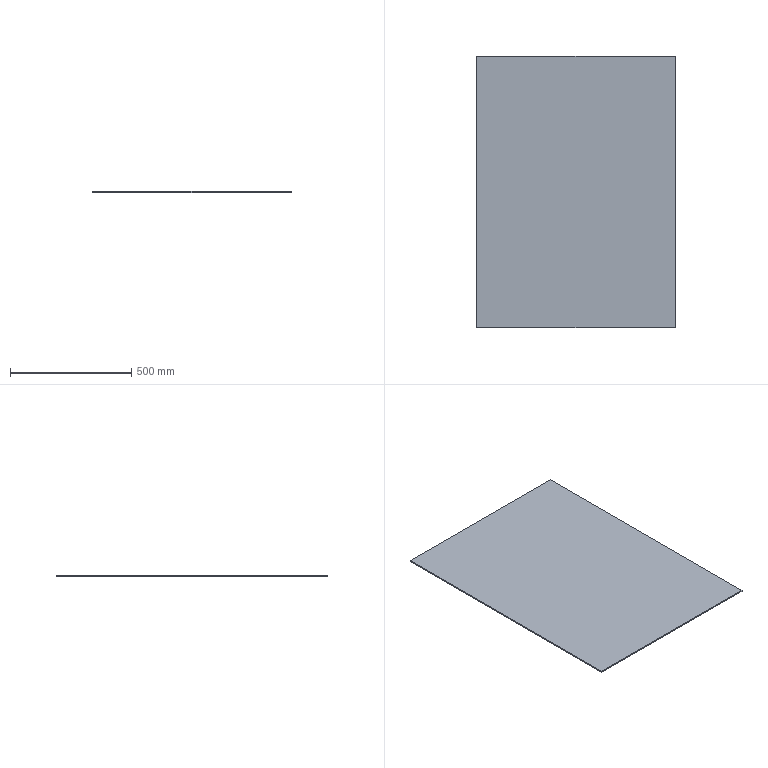Part | SolidWorks | features Extrusion 1 | 1 solid | 6 faces | box 818 x 1119 x 5 mm | volume 4576710 mm3 | plane 6
STEP:
#1=CARTESIAN_POINT('',(409.,-559.5,0.));
#2=VERTEX_POINT('',#1);
#3=CARTESIAN_POINT('',(409.,559.5,0.));
#4=VERTEX_POINT('',#3);
#5=CARTESIAN_POINT('',(409.,559.5,0.));
#6=DIRECTION('',(0.,1.,0.));
#7=VECTOR('',#6,1000.);
#8=LINE('',#5,#7);
#9=EDGE_CURVE('',#2,#4,#8,.T.);
#10=ORIENTED_EDGE('',*,*,#9,.T.);
#11=CARTESIAN_POINT('',(409.,559.5,5.));
#12=VERTEX_POINT('',#11);
#13=CARTESIAN_POINT('',(409.,559.5,5.));
#14=DIRECTION('',(0.,0.,-1.));
#15=VECTOR('',#14,1000.);
#16=LINE('',#13,#15);
#17=EDGE_CURVE('',#12,#4,#16,.T.);
#18=ORIENTED_EDGE('',*,*,#17,.F.);
#19=CARTESIAN_POINT('',(409.,-559.5,5.));
#20=VERTEX_POINT('',#19);
#21=CARTESIAN_POINT('',(409.,559.5,5.));
#22=DIRECTION('',(0.,1.,0.));
#23=VECTOR('',#22,1000.);
#24=LINE('',#21,#23);
#25=EDGE_CURVE('',#20,#12,#24,.T.);
#26=ORIENTED_EDGE('',*,*,#25,.F.);
#27=CARTESIAN_POINT('',(409.,-559.5,5.));
#28=DIRECTION('',(0.,0.,-1.));
#29=VECTOR('',#28,1000.);
#30=LINE('',#27,#29);
#31=EDGE_CURVE('',#20,#2,#30,.T.);
#32=ORIENTED_EDGE('',*,*,#31,.T.);
#33=EDGE_LOOP('',(#10,#18,#26,#32));
#34=FACE_OUTER_BOUND('',#33,.T.);
#35=CARTESIAN_POINT('',(409.,559.5,5.));
#36=DIRECTION('',(-1.,0.,0.));
#37=DIRECTION('',(0.,0.,1.));
#38=AXIS2_PLACEMENT_3D('',#35,#36,#37);
#39=PLANE('',#38);
#40=ADVANCED_FACE('',(#34),#39,.F.);
#41=CARTESIAN_POINT('',(-409.,559.5,0.));
#42=VERTEX_POINT('',#41);
#43=CARTESIAN_POINT('',(-409.,559.5,0.));
#44=DIRECTION('',(-1.,0.,0.));
#45=VECTOR('',#44,1000.);
#46=LINE('',#43,#45);
#47=EDGE_CURVE('',#4,#42,#46,.T.);
#48=ORIENTED_EDGE('',*,*,#47,.T.);
#49=CARTESIAN_POINT('',(-409.,559.5,5.));
#50=VERTEX_POINT('',#49);
#51=CARTESIAN_POINT('',(-409.,559.5,5.));
#52=DIRECTION('',(0.,0.,-1.));
#53=VECTOR('',#52,1000.);
#54=LINE('',#51,#53);
#55=EDGE_CURVE('',#50,#42,#54,.T.);
#56=ORIENTED_EDGE('',*,*,#55,.F.);
#57=CARTESIAN_POINT('',(-409.,559.5,5.));
#58=DIRECTION('',(-1.,0.,0.));
#59=VECTOR('',#58,1000.);
#60=LINE('',#57,#59);
#61=EDGE_CURVE('',#12,#50,#60,.T.);
#62=ORIENTED_EDGE('',*,*,#61,.F.);
#63=ORIENTED_EDGE('',*,*,#17,.T.);
#64=EDGE_LOOP('',(#48,#56,#62,#63));
#65=FACE_OUTER_BOUND('',#64,.T.);
#66=CARTESIAN_POINT('',(-409.,559.5,5.));
#67=DIRECTION('',(0.,-1.,0.));
#68=DIRECTION('',(0.,0.,-1.));
#69=AXIS2_PLACEMENT_3D('',#66,#67,#68);
#70=PLANE('',#69);
#71=ADVANCED_FACE('',(#65),#70,.F.);
#72=CARTESIAN_POINT('',(-409.,-559.5,0.));
#73=VERTEX_POINT('',#72);
#74=CARTESIAN_POINT('',(-409.,559.5,0.));
#75=DIRECTION('',(0.,-1.,0.));
#76=VECTOR('',#75,1000.);
#77=LINE('',#74,#76);
#78=EDGE_CURVE('',#42,#73,#77,.T.);
#79=ORIENTED_EDGE('',*,*,#78,.T.);
#80=CARTESIAN_POINT('',(-409.,-559.5,5.));
#81=VERTEX_POINT('',#80);
#82=CARTESIAN_POINT('',(-409.,-559.5,5.));
#83=DIRECTION('',(0.,0.,-1.));
#84=VECTOR('',#83,1000.);
#85=LINE('',#82,#84);
#86=EDGE_CURVE('',#81,#73,#85,.T.);
#87=ORIENTED_EDGE('',*,*,#86,.F.);
#88=CARTESIAN_POINT('',(-409.,559.5,5.));
#89=DIRECTION('',(0.,-1.,0.));
#90=VECTOR('',#89,1000.);
#91=LINE('',#88,#90);
#92=EDGE_CURVE('',#50,#81,#91,.T.);
#93=ORIENTED_EDGE('',*,*,#92,.F.);
#94=ORIENTED_EDGE('',*,*,#55,.T.);
#95=EDGE_LOOP('',(#79,#87,#93,#94));
#96=FACE_OUTER_BOUND('',#95,.T.);
#97=CARTESIAN_POINT('',(-409.,559.5,5.));
#98=DIRECTION('',(1.,0.,0.));
#99=DIRECTION('',(0.,0.,-1.));
#100=AXIS2_PLACEMENT_3D('',#97,#98,#99);
#101=PLANE('',#100);
#102=ADVANCED_FACE('',(#96),#101,.F.);
#103=CARTESIAN_POINT('',(-409.,-559.5,0.));
#104=DIRECTION('',(1.,0.,0.));
#105=VECTOR('',#104,1000.);
#106=LINE('',#103,#105);
#107=EDGE_CURVE('',#73,#2,#106,.T.);
#108=ORIENTED_EDGE('',*,*,#107,.T.);
#109=ORIENTED_EDGE('',*,*,#31,.F.);
#110=CARTESIAN_POINT('',(-409.,-559.5,5.));
#111=DIRECTION('',(1.,0.,0.));
#112=VECTOR('',#111,1000.);
#113=LINE('',#110,#112);
#114=EDGE_CURVE('',#81,#20,#113,.T.);
#115=ORIENTED_EDGE('',*,*,#114,.F.);
#116=ORIENTED_EDGE('',*,*,#86,.T.);
#117=EDGE_LOOP('',(#108,#109,#115,#116));
#118=FACE_OUTER_BOUND('',#117,.T.);
#119=CARTESIAN_POINT('',(-409.,-559.5,5.));
#120=DIRECTION('',(0.,1.,0.));
#121=DIRECTION('',(0.,0.,1.));
#122=AXIS2_PLACEMENT_3D('',#119,#120,#121);
#123=PLANE('',#122);
#124=ADVANCED_FACE('',(#118),#123,.F.);
#125=ORIENTED_EDGE('',*,*,#25,.T.);
#126=ORIENTED_EDGE('',*,*,#61,.T.);
#127=ORIENTED_EDGE('',*,*,#92,.T.);
#128=ORIENTED_EDGE('',*,*,#114,.T.);
#129=EDGE_LOOP('',(#125,#126,#127,#128));
#130=FACE_OUTER_BOUND('',#129,.T.);
#131=CARTESIAN_POINT('',(0.,0.,5.));
#132=DIRECTION('',(0.,0.,1.));
#133=DIRECTION('',(1.,0.,0.));
#134=AXIS2_PLACEMENT_3D('',#131,#132,#133);
#135=PLANE('',#134);
#136=ADVANCED_FACE('',(#130),#135,.T.);
#137=ORIENTED_EDGE('',*,*,#9,.F.);
#138=ORIENTED_EDGE('',*,*,#107,.F.);
#139=ORIENTED_EDGE('',*,*,#78,.F.);
#140=ORIENTED_EDGE('',*,*,#47,.F.);
#141=EDGE_LOOP('',(#137,#138,#139,#140));
#142=FACE_OUTER_BOUND('',#141,.T.);
#143=CARTESIAN_POINT('',(0.,0.,0.));
#144=DIRECTION('',(0.,0.,1.));
#145=DIRECTION('',(1.,0.,0.));
#146=AXIS2_PLACEMENT_3D('',#143,#144,#145);
#147=PLANE('',#146);
#148=ADVANCED_FACE('',(#142),#147,.F.);
#149=CLOSED_SHELL('',(#40,#71,#102,#124,#136,#148));
#150=MANIFOLD_SOLID_BREP('',#149);
#151=CARTESIAN_POINT('',(0.,0.,0.));
#152=DIRECTION('',(0.,0.,1.));
#153=DIRECTION('',(1.,0.,0.));
#154=AXIS2_PLACEMENT_3D('',#151,#152,#153);
#155=(LENGTH_UNIT()NAMED_UNIT(*)SI_UNIT(.MILLI.,.METRE.));
#156=UNCERTAINTY_MEASURE_WITH_UNIT(LENGTH_MEASURE(0.00001),#155,'','');
#157=(NAMED_UNIT(*)PLANE_ANGLE_UNIT()SI_UNIT($,.RADIAN.));
#158=(NAMED_UNIT(*)SI_UNIT($,.STERADIAN.)SOLID_ANGLE_UNIT());
#159=(GEOMETRIC_REPRESENTATION_CONTEXT(3)GLOBAL_UNCERTAINTY_ASSIGNED_CONTEXT((#156))GLOBAL_UNIT_ASSIGNED_CONTEXT((#155,#157,#158))REPRESENTATION_CONTEXT('',''));
#160=ADVANCED_BREP_SHAPE_REPRESENTATION('',(#150,#154),#159);